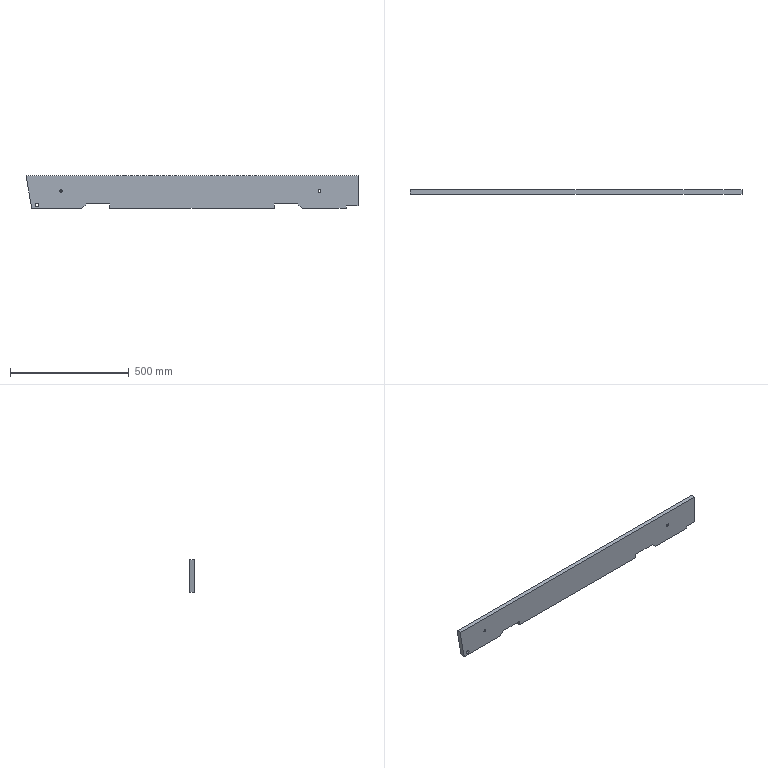Part | STEP file | Frame_right | 1 solid | 19 faces | box 1400 x 18 x 137 mm | volume 3336381 mm3 | plane 16 | cylinder 3 | commonest cylinder face diameters 11 x2 15 x1
STEP:
#1=CARTESIAN_POINT('',(0.,0.,0.));
#2=DIRECTION('',(0.,0.,1.));
#3=DIRECTION('',(1.,0.,0.));
#4=AXIS2_PLACEMENT_3D('',#1,#2,#3);
#5=CARTESIAN_POINT('',(-675.843,0.,-68.5));
#6=VERTEX_POINT('',#5);
#7=CARTESIAN_POINT('',(-464.5,0.,-68.5));
#8=VERTEX_POINT('',#7);
#9=CARTESIAN_POINT('',(-700.,0.,-68.5));
#10=DIRECTION('',(1.,0.,0.));
#11=VECTOR('',#10,1.);
#12=LINE('',#9,#11);
#13=CARTESIAN_POINT('',(-700.,0.,-68.5));
#14=DIRECTION('',(0.,0.,1.));
#15=DIRECTION('',(1.,0.,0.));
#16=AXIS2_PLACEMENT_3D('',#13,#14,#15);
#17=PLANE('',#16);
#18=CARTESIAN_POINT('',(0.,0.));
#19=DIRECTION('',(1.,0.));
#20=VECTOR('',#19,1.);
#21=LINE('',#18,#20);
#22=(GEOMETRIC_REPRESENTATION_CONTEXT(2)PARAMETRIC_REPRESENTATION_CONTEXT()REPRESENTATION_CONTEXT('',''));
#23=DEFINITIONAL_REPRESENTATION('',(#21),#22);
#24=PCURVE('',#17,#23);
#25=CARTESIAN_POINT('',(0.,0.,0.));
#26=DIRECTION('',(0.,1.,0.));
#27=DIRECTION('',(0.,0.,1.));
#28=AXIS2_PLACEMENT_3D('',#25,#26,#27);
#29=PLANE('',#28);
#30=CARTESIAN_POINT('',(-68.5,-700.));
#31=DIRECTION('',(0.,1.));
#32=VECTOR('',#31,1.);
#33=LINE('',#30,#32);
#34=(GEOMETRIC_REPRESENTATION_CONTEXT(2)PARAMETRIC_REPRESENTATION_CONTEXT()REPRESENTATION_CONTEXT('',''));
#35=DEFINITIONAL_REPRESENTATION('',(#33),#34);
#36=PCURVE('',#29,#35);
#37=SURFACE_CURVE('',#12,(#24,#36),.PCURVE_S1.);
#38=EDGE_CURVE('',#6,#8,#37,.T.);
#39=ORIENTED_EDGE('',*,*,#38,.F.);
#40=CARTESIAN_POINT('',(-675.843,-18.,-68.5));
#41=VERTEX_POINT('',#40);
#42=CARTESIAN_POINT('',(-675.843,0.,-68.5));
#43=DIRECTION('',(0.,-1.,0.));
#44=VECTOR('',#43,1.);
#45=LINE('',#42,#44);
#46=CARTESIAN_POINT('',(24.157,0.));
#47=DIRECTION('',(0.,-1.));
#48=VECTOR('',#47,1.);
#49=LINE('',#46,#48);
#50=(GEOMETRIC_REPRESENTATION_CONTEXT(2)PARAMETRIC_REPRESENTATION_CONTEXT()REPRESENTATION_CONTEXT('',''));
#51=DEFINITIONAL_REPRESENTATION('',(#49),#50);
#52=PCURVE('',#17,#51);
#53=CARTESIAN_POINT('',(-700.,0.,68.5));
#54=DIRECTION('',(0.9848,0.,0.1736));
#55=DIRECTION('',(0.1736,0.,-0.9848));
#56=AXIS2_PLACEMENT_3D('',#53,#54,#55);
#57=PLANE('',#56);
#58=CARTESIAN_POINT('',(139.113,0.));
#59=DIRECTION('',(0.,-1.));
#60=VECTOR('',#59,1.);
#61=LINE('',#58,#60);
#62=(GEOMETRIC_REPRESENTATION_CONTEXT(2)PARAMETRIC_REPRESENTATION_CONTEXT()REPRESENTATION_CONTEXT('',''));
#63=DEFINITIONAL_REPRESENTATION('',(#61),#62);
#64=PCURVE('',#57,#63);
#65=SURFACE_CURVE('',#45,(#52,#64),.PCURVE_S1.);
#66=EDGE_CURVE('',#6,#41,#65,.T.);
#67=ORIENTED_EDGE('',*,*,#66,.T.);
#68=CARTESIAN_POINT('',(-464.5,-18.,-68.5));
#69=VERTEX_POINT('',#68);
#70=CARTESIAN_POINT('',(-700.,-18.,-68.5));
#71=DIRECTION('',(1.,0.,0.));
#72=VECTOR('',#71,1.);
#73=LINE('',#70,#72);
#74=CARTESIAN_POINT('',(0.,-18.));
#75=DIRECTION('',(1.,0.));
#76=VECTOR('',#75,1.);
#77=LINE('',#74,#76);
#78=(GEOMETRIC_REPRESENTATION_CONTEXT(2)PARAMETRIC_REPRESENTATION_CONTEXT()REPRESENTATION_CONTEXT('',''));
#79=DEFINITIONAL_REPRESENTATION('',(#77),#78);
#80=PCURVE('',#17,#79);
#81=CARTESIAN_POINT('',(0.,-18.,0.));
#82=DIRECTION('',(0.,1.,0.));
#83=DIRECTION('',(0.,0.,1.));
#84=AXIS2_PLACEMENT_3D('',#81,#82,#83);
#85=PLANE('',#84);
#86=CARTESIAN_POINT('',(-68.5,-700.));
#87=DIRECTION('',(0.,1.));
#88=VECTOR('',#87,1.);
#89=LINE('',#86,#88);
#90=(GEOMETRIC_REPRESENTATION_CONTEXT(2)PARAMETRIC_REPRESENTATION_CONTEXT()REPRESENTATION_CONTEXT('',''));
#91=DEFINITIONAL_REPRESENTATION('',(#89),#90);
#92=PCURVE('',#85,#91);
#93=SURFACE_CURVE('',#73,(#80,#92),.PCURVE_S1.);
#94=EDGE_CURVE('',#41,#69,#93,.T.);
#95=ORIENTED_EDGE('',*,*,#94,.T.);
#96=CARTESIAN_POINT('',(-464.5,-18.,-68.5));
#97=DIRECTION('',(0.,1.,0.));
#98=VECTOR('',#97,1.);
#99=LINE('',#96,#98);
#100=CARTESIAN_POINT('',(235.5,-18.));
#101=DIRECTION('',(0.,1.));
#102=VECTOR('',#101,1.);
#103=LINE('',#100,#102);
#104=(GEOMETRIC_REPRESENTATION_CONTEXT(2)PARAMETRIC_REPRESENTATION_CONTEXT()REPRESENTATION_CONTEXT('',''));
#105=DEFINITIONAL_REPRESENTATION('',(#103),#104);
#106=PCURVE('',#17,#105);
#107=CARTESIAN_POINT('',(-446.5,-18.,-50.5));
#108=DIRECTION('',(-0.7071,0.,0.7071));
#109=DIRECTION('',(-0.7071,0.,-0.7071));
#110=AXIS2_PLACEMENT_3D('',#107,#108,#109);
#111=PLANE('',#110);
#112=CARTESIAN_POINT('',(25.456,0.));
#113=DIRECTION('',(0.,-1.));
#114=VECTOR('',#113,1.);
#115=LINE('',#112,#114);
#116=(GEOMETRIC_REPRESENTATION_CONTEXT(2)PARAMETRIC_REPRESENTATION_CONTEXT()REPRESENTATION_CONTEXT('',''));
#117=DEFINITIONAL_REPRESENTATION('',(#115),#116);
#118=PCURVE('',#111,#117);
#119=SURFACE_CURVE('',#99,(#106,#118),.PCURVE_S1.);
#120=EDGE_CURVE('',#69,#8,#119,.T.);
#121=ORIENTED_EDGE('',*,*,#120,.T.);
#122=EDGE_LOOP('',(#39,#67,#95,#121));
#123=FACE_BOUND('',#122,.F.);
#124=ADVANCED_FACE('',(#123),#17,.F.);
#125=ORIENTED_EDGE('',*,*,#38,.F.);
#126=CARTESIAN_POINT('',(-700.,0.,68.5));
#127=VERTEX_POINT('',#126);
#128=CARTESIAN_POINT('',(-683.589,0.,-24.571));
#129=DIRECTION('',(0.1736,0.,-0.9848));
#130=VECTOR('',#129,1.);
#131=LINE('',#128,#130);
#132=CARTESIAN_POINT('',(-24.571,-683.589));
#133=DIRECTION('',(-0.9848,0.1736));
#134=VECTOR('',#133,1.);
#135=LINE('',#132,#134);
#136=(GEOMETRIC_REPRESENTATION_CONTEXT(2)PARAMETRIC_REPRESENTATION_CONTEXT()REPRESENTATION_CONTEXT('',''));
#137=DEFINITIONAL_REPRESENTATION('',(#135),#136);
#138=PCURVE('',#29,#137);
#139=CARTESIAN_POINT('',(94.507,0.));
#140=DIRECTION('',(1.,0.));
#141=VECTOR('',#140,1.);
#142=LINE('',#139,#141);
#143=(GEOMETRIC_REPRESENTATION_CONTEXT(2)PARAMETRIC_REPRESENTATION_CONTEXT()REPRESENTATION_CONTEXT('',''));
#144=DEFINITIONAL_REPRESENTATION('',(#142),#143);
#145=PCURVE('',#57,#144);
#146=SURFACE_CURVE('',#131,(#138,#145),.PCURVE_S1.);
#147=EDGE_CURVE('',#127,#6,#146,.T.);
#148=ORIENTED_EDGE('',*,*,#147,.F.);
#149=CARTESIAN_POINT('',(700.,0.,68.5));
#150=VERTEX_POINT('',#149);
#151=CARTESIAN_POINT('',(700.,0.,68.5));
#152=DIRECTION('',(-1.,0.,0.));
#153=VECTOR('',#152,1.);
#154=LINE('',#151,#153);
#155=CARTESIAN_POINT('',(68.5,700.));
#156=DIRECTION('',(0.,-1.));
#157=VECTOR('',#156,1.);
#158=LINE('',#155,#157);
#159=(GEOMETRIC_REPRESENTATION_CONTEXT(2)PARAMETRIC_REPRESENTATION_CONTEXT()REPRESENTATION_CONTEXT('',''));
#160=DEFINITIONAL_REPRESENTATION('',(#158),#159);
#161=PCURVE('',#29,#160);
#162=CARTESIAN_POINT('',(700.,0.,68.5));
#163=DIRECTION('',(0.,0.,-1.));
#164=DIRECTION('',(-1.,0.,0.));
#165=AXIS2_PLACEMENT_3D('',#162,#163,#164);
#166=PLANE('',#165);
#167=CARTESIAN_POINT('',(0.,0.));
#168=DIRECTION('',(1.,0.));
#169=VECTOR('',#168,1.);
#170=LINE('',#167,#169);
#171=(GEOMETRIC_REPRESENTATION_CONTEXT(2)PARAMETRIC_REPRESENTATION_CONTEXT()REPRESENTATION_CONTEXT('',''));
#172=DEFINITIONAL_REPRESENTATION('',(#170),#171);
#173=PCURVE('',#166,#172);
#174=SURFACE_CURVE('',#154,(#161,#173),.PCURVE_S1.);
#175=EDGE_CURVE('',#150,#127,#174,.T.);
#176=ORIENTED_EDGE('',*,*,#175,.F.);
#177=CARTESIAN_POINT('',(700.,0.,-58.5));
#178=VERTEX_POINT('',#177);
#179=CARTESIAN_POINT('',(700.,0.,-68.5));
#180=DIRECTION('',(0.,0.,1.));
#181=VECTOR('',#180,1.);
#182=LINE('',#179,#181);
#183=CARTESIAN_POINT('',(-68.5,700.));
#184=DIRECTION('',(1.,0.));
#185=VECTOR('',#184,1.);
#186=LINE('',#183,#185);
#187=(GEOMETRIC_REPRESENTATION_CONTEXT(2)PARAMETRIC_REPRESENTATION_CONTEXT()REPRESENTATION_CONTEXT('',''));
#188=DEFINITIONAL_REPRESENTATION('',(#186),#187);
#189=PCURVE('',#29,#188);
#190=CARTESIAN_POINT('',(700.,0.,-68.5));
#191=DIRECTION('',(-1.,0.,0.));
#192=DIRECTION('',(0.,0.,1.));
#193=AXIS2_PLACEMENT_3D('',#190,#191,#192);
#194=PLANE('',#193);
#195=CARTESIAN_POINT('',(0.,0.));
#196=DIRECTION('',(1.,0.));
#197=VECTOR('',#196,1.);
#198=LINE('',#195,#197);
#199=(GEOMETRIC_REPRESENTATION_CONTEXT(2)PARAMETRIC_REPRESENTATION_CONTEXT()REPRESENTATION_CONTEXT('',''));
#200=DEFINITIONAL_REPRESENTATION('',(#198),#199);
#201=PCURVE('',#194,#200);
#202=SURFACE_CURVE('',#182,(#189,#201),.PCURVE_S1.);
#203=EDGE_CURVE('',#178,#150,#202,.T.);
#204=ORIENTED_EDGE('',*,*,#203,.F.);
#205=CARTESIAN_POINT('',(650.,0.,-58.5));
#206=VERTEX_POINT('',#205);
#207=CARTESIAN_POINT('',(350.,0.,-58.5));
#208=DIRECTION('',(1.,0.,0.));
#209=VECTOR('',#208,1.);
#210=LINE('',#207,#209);
#211=CARTESIAN_POINT('',(-58.5,350.));
#212=DIRECTION('',(0.,1.));
#213=VECTOR('',#212,1.);
#214=LINE('',#211,#213);
#215=(GEOMETRIC_REPRESENTATION_CONTEXT(2)PARAMETRIC_REPRESENTATION_CONTEXT()REPRESENTATION_CONTEXT('',''));
#216=DEFINITIONAL_REPRESENTATION('',(#214),#215);
#217=PCURVE('',#29,#216);
#218=CARTESIAN_POINT('',(700.,-18.,-58.5));
#219=DIRECTION('',(0.,0.,1.));
#220=DIRECTION('',(-1.,0.,0.));
#221=AXIS2_PLACEMENT_3D('',#218,#219,#220);
#222=PLANE('',#221);
#223=CARTESIAN_POINT('',(350.,-18.));
#224=DIRECTION('',(-1.,0.));
#225=VECTOR('',#224,1.);
#226=LINE('',#223,#225);
#227=(GEOMETRIC_REPRESENTATION_CONTEXT(2)PARAMETRIC_REPRESENTATION_CONTEXT()REPRESENTATION_CONTEXT('',''));
#228=DEFINITIONAL_REPRESENTATION('',(#226),#227);
#229=PCURVE('',#222,#228);
#230=SURFACE_CURVE('',#210,(#217,#229),.PCURVE_S1.);
#231=EDGE_CURVE('',#206,#178,#230,.T.);
#232=ORIENTED_EDGE('',*,*,#231,.F.);
#233=CARTESIAN_POINT('',(650.,0.,-68.5));
#234=VERTEX_POINT('',#233);
#235=CARTESIAN_POINT('',(650.,0.,-29.25));
#236=DIRECTION('',(0.,0.,1.));
#237=VECTOR('',#236,1.);
#238=LINE('',#235,#237);
#239=CARTESIAN_POINT('',(-29.25,650.));
#240=DIRECTION('',(1.,0.));
#241=VECTOR('',#240,1.);
#242=LINE('',#239,#241);
#243=(GEOMETRIC_REPRESENTATION_CONTEXT(2)PARAMETRIC_REPRESENTATION_CONTEXT()REPRESENTATION_CONTEXT('',''));
#244=DEFINITIONAL_REPRESENTATION('',(#242),#243);
#245=PCURVE('',#29,#244);
#246=CARTESIAN_POINT('',(650.,-18.,-58.5));
#247=DIRECTION('',(-1.,0.,0.));
#248=DIRECTION('',(0.,0.,-1.));
#249=AXIS2_PLACEMENT_3D('',#246,#247,#248);
#250=PLANE('',#249);
#251=CARTESIAN_POINT('',(-29.25,-18.));
#252=DIRECTION('',(-1.,0.));
#253=VECTOR('',#252,1.);
#254=LINE('',#251,#253);
#255=(GEOMETRIC_REPRESENTATION_CONTEXT(2)PARAMETRIC_REPRESENTATION_CONTEXT()REPRESENTATION_CONTEXT('',''));
#256=DEFINITIONAL_REPRESENTATION('',(#254),#255);
#257=PCURVE('',#250,#256);
#258=SURFACE_CURVE('',#238,(#245,#257),.PCURVE_S1.);
#259=EDGE_CURVE('',#234,#206,#258,.T.);
#260=ORIENTED_EDGE('',*,*,#259,.F.);
#261=CARTESIAN_POINT('',(464.5,0.,-68.5));
#262=VERTEX_POINT('',#261);
#263=CARTESIAN_POINT('',(-700.,0.,-68.5));
#264=DIRECTION('',(1.,0.,0.));
#265=VECTOR('',#264,1.);
#266=LINE('',#263,#265);
#267=CARTESIAN_POINT('',(-68.5,-700.));
#268=DIRECTION('',(0.,1.));
#269=VECTOR('',#268,1.);
#270=LINE('',#267,#269);
#271=(GEOMETRIC_REPRESENTATION_CONTEXT(2)PARAMETRIC_REPRESENTATION_CONTEXT()REPRESENTATION_CONTEXT('',''));
#272=DEFINITIONAL_REPRESENTATION('',(#270),#271);
#273=PCURVE('',#29,#272);
#274=CARTESIAN_POINT('',(-700.,0.,-68.5));
#275=DIRECTION('',(0.,0.,1.));
#276=DIRECTION('',(1.,0.,0.));
#277=AXIS2_PLACEMENT_3D('',#274,#275,#276);
#278=PLANE('',#277);
#279=CARTESIAN_POINT('',(0.,0.));
#280=DIRECTION('',(1.,0.));
#281=VECTOR('',#280,1.);
#282=LINE('',#279,#281);
#283=(GEOMETRIC_REPRESENTATION_CONTEXT(2)PARAMETRIC_REPRESENTATION_CONTEXT()REPRESENTATION_CONTEXT('',''));
#284=DEFINITIONAL_REPRESENTATION('',(#282),#283);
#285=PCURVE('',#278,#284);
#286=SURFACE_CURVE('',#266,(#273,#285),.PCURVE_S1.);
#287=EDGE_CURVE('',#262,#234,#286,.T.);
#288=ORIENTED_EDGE('',*,*,#287,.F.);
#289=CARTESIAN_POINT('',(446.5,0.,-50.5));
#290=VERTEX_POINT('',#289);
#291=CARTESIAN_POINT('',(322.25,0.,73.75));
#292=DIRECTION('',(-0.7071,0.,0.7071));
#293=VECTOR('',#292,1.);
#294=LINE('',#291,#293);
#295=CARTESIAN_POINT('',(73.75,322.25));
#296=DIRECTION('',(0.7071,-0.7071));
#297=VECTOR('',#296,1.);
#298=LINE('',#295,#297);
#299=(GEOMETRIC_REPRESENTATION_CONTEXT(2)PARAMETRIC_REPRESENTATION_CONTEXT()REPRESENTATION_CONTEXT('',''));
#300=DEFINITIONAL_REPRESENTATION('',(#298),#299);
#301=PCURVE('',#29,#300);
#302=CARTESIAN_POINT('',(446.5,-18.,-50.5));
#303=DIRECTION('',(-0.7071,0.,-0.7071));
#304=DIRECTION('',(0.7071,0.,-0.7071));
#305=AXIS2_PLACEMENT_3D('',#302,#303,#304);
#306=PLANE('',#305);
#307=CARTESIAN_POINT('',(-175.716,-18.));
#308=DIRECTION('',(-1.,0.));
#309=VECTOR('',#308,1.);
#310=LINE('',#307,#309);
#311=(GEOMETRIC_REPRESENTATION_CONTEXT(2)PARAMETRIC_REPRESENTATION_CONTEXT()REPRESENTATION_CONTEXT('',''));
#312=DEFINITIONAL_REPRESENTATION('',(#310),#311);
#313=PCURVE('',#306,#312);
#314=SURFACE_CURVE('',#294,(#301,#313),.PCURVE_S1.);
#315=EDGE_CURVE('',#262,#290,#314,.T.);
#316=ORIENTED_EDGE('',*,*,#315,.T.);
#317=CARTESIAN_POINT('',(346.5,0.,-50.5));
#318=VERTEX_POINT('',#317);
#319=CARTESIAN_POINT('',(173.25,0.,-50.5));
#320=DIRECTION('',(-1.,0.,0.));
#321=VECTOR('',#320,1.);
#322=LINE('',#319,#321);
#323=CARTESIAN_POINT('',(-50.5,173.25));
#324=DIRECTION('',(0.,-1.));
#325=VECTOR('',#324,1.);
#326=LINE('',#323,#325);
#327=(GEOMETRIC_REPRESENTATION_CONTEXT(2)PARAMETRIC_REPRESENTATION_CONTEXT()REPRESENTATION_CONTEXT('',''));
#328=DEFINITIONAL_REPRESENTATION('',(#326),#327);
#329=PCURVE('',#29,#328);
#330=CARTESIAN_POINT('',(346.5,-18.,-50.5));
#331=DIRECTION('',(0.,0.,-1.));
#332=DIRECTION('',(1.,0.,0.));
#333=AXIS2_PLACEMENT_3D('',#330,#331,#332);
#334=PLANE('',#333);
#335=CARTESIAN_POINT('',(-173.25,-18.));
#336=DIRECTION('',(-1.,0.));
#337=VECTOR('',#336,1.);
#338=LINE('',#335,#337);
#339=(GEOMETRIC_REPRESENTATION_CONTEXT(2)PARAMETRIC_REPRESENTATION_CONTEXT()REPRESENTATION_CONTEXT('',''));
#340=DEFINITIONAL_REPRESENTATION('',(#338),#339);
#341=PCURVE('',#334,#340);
#342=SURFACE_CURVE('',#322,(#329,#341),.PCURVE_S1.);
#343=EDGE_CURVE('',#290,#318,#342,.T.);
#344=ORIENTED_EDGE('',*,*,#343,.T.);
#345=CARTESIAN_POINT('',(346.5,0.,-68.5));
#346=VERTEX_POINT('',#345);
#347=CARTESIAN_POINT('',(346.5,0.,-34.25));
#348=DIRECTION('',(0.,0.,-1.));
#349=VECTOR('',#348,1.);
#350=LINE('',#347,#349);
#351=CARTESIAN_POINT('',(-34.25,346.5));
#352=DIRECTION('',(-1.,0.));
#353=VECTOR('',#352,1.);
#354=LINE('',#351,#353);
#355=(GEOMETRIC_REPRESENTATION_CONTEXT(2)PARAMETRIC_REPRESENTATION_CONTEXT()REPRESENTATION_CONTEXT('',''));
#356=DEFINITIONAL_REPRESENTATION('',(#354),#355);
#357=PCURVE('',#29,#356);
#358=CARTESIAN_POINT('',(346.5,-18.,-68.5));
#359=DIRECTION('',(1.,0.,0.));
#360=DIRECTION('',(0.,0.,1.));
#361=AXIS2_PLACEMENT_3D('',#358,#359,#360);
#362=PLANE('',#361);
#363=CARTESIAN_POINT('',(34.25,-18.));
#364=DIRECTION('',(-1.,0.));
#365=VECTOR('',#364,1.);
#366=LINE('',#363,#365);
#367=(GEOMETRIC_REPRESENTATION_CONTEXT(2)PARAMETRIC_REPRESENTATION_CONTEXT()REPRESENTATION_CONTEXT('',''));
#368=DEFINITIONAL_REPRESENTATION('',(#366),#367);
#369=PCURVE('',#362,#368);
#370=SURFACE_CURVE('',#350,(#357,#369),.PCURVE_S1.);
#371=EDGE_CURVE('',#318,#346,#370,.T.);
#372=ORIENTED_EDGE('',*,*,#371,.T.);
#373=CARTESIAN_POINT('',(-346.5,0.,-68.5));
#374=VERTEX_POINT('',#373);
#375=CARTESIAN_POINT('',(-700.,0.,-68.5));
#376=DIRECTION('',(1.,0.,0.));
#377=VECTOR('',#376,1.);
#378=LINE('',#375,#377);
#379=CARTESIAN_POINT('',(-68.5,-700.));
#380=DIRECTION('',(0.,1.));
#381=VECTOR('',#380,1.);
#382=LINE('',#379,#381);
#383=(GEOMETRIC_REPRESENTATION_CONTEXT(2)PARAMETRIC_REPRESENTATION_CONTEXT()REPRESENTATION_CONTEXT('',''));
#384=DEFINITIONAL_REPRESENTATION('',(#382),#383);
#385=PCURVE('',#29,#384);
#386=CARTESIAN_POINT('',(-700.,0.,-68.5));
#387=DIRECTION('',(0.,0.,1.));
#388=DIRECTION('',(1.,0.,0.));
#389=AXIS2_PLACEMENT_3D('',#386,#387,#388);
#390=PLANE('',#389);
#391=CARTESIAN_POINT('',(0.,0.));
#392=DIRECTION('',(1.,0.));
#393=VECTOR('',#392,1.);
#394=LINE('',#391,#393);
#395=(GEOMETRIC_REPRESENTATION_CONTEXT(2)PARAMETRIC_REPRESENTATION_CONTEXT()REPRESENTATION_CONTEXT('',''));
#396=DEFINITIONAL_REPRESENTATION('',(#394),#395);
#397=PCURVE('',#390,#396);
#398=SURFACE_CURVE('',#378,(#385,#397),.PCURVE_S1.);
#399=EDGE_CURVE('',#374,#346,#398,.T.);
#400=ORIENTED_EDGE('',*,*,#399,.F.);
#401=CARTESIAN_POINT('',(-346.5,0.,-50.5));
#402=VERTEX_POINT('',#401);
#403=CARTESIAN_POINT('',(-346.5,0.,-34.25));
#404=DIRECTION('',(0.,0.,-1.));
#405=VECTOR('',#404,1.);
#406=LINE('',#403,#405);
#407=CARTESIAN_POINT('',(-34.25,-346.5));
#408=DIRECTION('',(-1.,0.));
#409=VECTOR('',#408,1.);
#410=LINE('',#407,#409);
#411=(GEOMETRIC_REPRESENTATION_CONTEXT(2)PARAMETRIC_REPRESENTATION_CONTEXT()REPRESENTATION_CONTEXT('',''));
#412=DEFINITIONAL_REPRESENTATION('',(#410),#411);
#413=PCURVE('',#29,#412);
#414=CARTESIAN_POINT('',(-346.5,-18.,-68.5));
#415=DIRECTION('',(1.,0.,0.));
#416=DIRECTION('',(0.,0.,1.));
#417=AXIS2_PLACEMENT_3D('',#414,#415,#416);
#418=PLANE('',#417);
#419=CARTESIAN_POINT('',(34.25,-18.));
#420=DIRECTION('',(-1.,0.));
#421=VECTOR('',#420,1.);
#422=LINE('',#419,#421);
#423=(GEOMETRIC_REPRESENTATION_CONTEXT(2)PARAMETRIC_REPRESENTATION_CONTEXT()REPRESENTATION_CONTEXT('',''));
#424=DEFINITIONAL_REPRESENTATION('',(#422),#423);
#425=PCURVE('',#418,#424);
#426=SURFACE_CURVE('',#406,(#413,#425),.PCURVE_S1.);
#427=EDGE_CURVE('',#402,#374,#426,.T.);
#428=ORIENTED_EDGE('',*,*,#427,.F.);
#429=CARTESIAN_POINT('',(-446.5,0.,-50.5));
#430=VERTEX_POINT('',#429);
#431=CARTESIAN_POINT('',(-173.25,0.,-50.5));
#432=DIRECTION('',(1.,0.,0.));
#433=VECTOR('',#432,1.);
#434=LINE('',#431,#433);
#435=CARTESIAN_POINT('',(-50.5,-173.25));
#436=DIRECTION('',(0.,1.));
#437=VECTOR('',#436,1.);
#438=LINE('',#435,#437);
#439=(GEOMETRIC_REPRESENTATION_CONTEXT(2)PARAMETRIC_REPRESENTATION_CONTEXT()REPRESENTATION_CONTEXT('',''));
#440=DEFINITIONAL_REPRESENTATION('',(#438),#439);
#441=PCURVE('',#29,#440);
#442=CARTESIAN_POINT('',(-346.5,-18.,-50.5));
#443=DIRECTION('',(0.,0.,1.));
#444=DIRECTION('',(-1.,0.,0.));
#445=AXIS2_PLACEMENT_3D('',#442,#443,#444);
#446=PLANE('',#445);
#447=CARTESIAN_POINT('',(-173.25,-18.));
#448=DIRECTION('',(-1.,0.));
#449=VECTOR('',#448,1.);
#450=LINE('',#447,#449);
#451=(GEOMETRIC_REPRESENTATION_CONTEXT(2)PARAMETRIC_REPRESENTATION_CONTEXT()REPRESENTATION_CONTEXT('',''));
#452=DEFINITIONAL_REPRESENTATION('',(#450),#451);
#453=PCURVE('',#446,#452);
#454=SURFACE_CURVE('',#434,(#441,#453),.PCURVE_S1.);
#455=EDGE_CURVE('',#430,#402,#454,.T.);
#456=ORIENTED_EDGE('',*,*,#455,.F.);
#457=CARTESIAN_POINT('',(-322.25,0.,73.75));
#458=DIRECTION('',(0.7071,0.,0.7071));
#459=VECTOR('',#458,1.);
#460=LINE('',#457,#459);
#461=CARTESIAN_POINT('',(73.75,-322.25));
#462=DIRECTION('',(0.7071,0.7071));
#463=VECTOR('',#462,1.);
#464=LINE('',#461,#463);
#465=(GEOMETRIC_REPRESENTATION_CONTEXT(2)PARAMETRIC_REPRESENTATION_CONTEXT()REPRESENTATION_CONTEXT('',''));
#466=DEFINITIONAL_REPRESENTATION('',(#464),#465);
#467=PCURVE('',#29,#466);
#468=CARTESIAN_POINT('',(-175.716,-18.));
#469=DIRECTION('',(-1.,0.));
#470=VECTOR('',#469,1.);
#471=LINE('',#468,#470);
#472=(GEOMETRIC_REPRESENTATION_CONTEXT(2)PARAMETRIC_REPRESENTATION_CONTEXT()REPRESENTATION_CONTEXT('',''));
#473=DEFINITIONAL_REPRESENTATION('',(#471),#472);
#474=PCURVE('',#111,#473);
#475=SURFACE_CURVE('',#460,(#467,#474),.PCURVE_S1.);
#476=EDGE_CURVE('',#8,#430,#475,.T.);
#477=ORIENTED_EDGE('',*,*,#476,.F.);
#478=EDGE_LOOP('',(#125,#148,#176,#204,#232,#260,#288,#316,#344,#372,#400,#428,#456,#477));
#479=FACE_BOUND('',#478,.T.);
#480=CARTESIAN_POINT('',(-661.343,0.,-55.5));
#481=VERTEX_POINT('',#480);
#482=CARTESIAN_POINT('',(-653.843,0.,-55.5));
#483=DIRECTION('',(0.,1.,0.));
#484=DIRECTION('',(-1.,0.,0.));
#485=AXIS2_PLACEMENT_3D('',#482,#483,#484);
#486=CIRCLE('',#485,7.5);
#487=CARTESIAN_POINT('',(-55.5,-653.843));
#488=DIRECTION('',(0.,-1.));
#489=AXIS2_PLACEMENT_2D('',#487,#488);
#490=CIRCLE('',#489,7.5);
#491=(GEOMETRIC_REPRESENTATION_CONTEXT(2)PARAMETRIC_REPRESENTATION_CONTEXT()REPRESENTATION_CONTEXT('',''));
#492=DEFINITIONAL_REPRESENTATION('',(#490),#491);
#493=PCURVE('',#29,#492);
#494=CARTESIAN_POINT('',(-653.843,-18.,-55.5));
#495=DIRECTION('',(0.,1.,0.));
#496=DIRECTION('',(-1.,0.,0.));
#497=AXIS2_PLACEMENT_3D('',#494,#495,#496);
#498=CYLINDRICAL_SURFACE('',#497,7.5);
#499=CARTESIAN_POINT('',(0.,18.));
#500=DIRECTION('',(1.,0.));
#501=VECTOR('',#500,1.);
#502=LINE('',#499,#501);
#503=(GEOMETRIC_REPRESENTATION_CONTEXT(2)PARAMETRIC_REPRESENTATION_CONTEXT()REPRESENTATION_CONTEXT('',''));
#504=DEFINITIONAL_REPRESENTATION('',(#502),#503);
#505=PCURVE('',#498,#504);
#506=SURFACE_CURVE('',#486,(#493,#505),.PCURVE_S1.);
#507=EDGE_CURVE('',#481,#481,#506,.T.);
#508=ORIENTED_EDGE('',*,*,#507,.F.);
#509=EDGE_LOOP('',(#508));
#510=FACE_BOUND('',#509,.T.);
#511=CARTESIAN_POINT('',(-557.9,0.,4.5));
#512=VERTEX_POINT('',#511);
#513=CARTESIAN_POINT('',(-552.4,0.,4.5));
#514=DIRECTION('',(0.,1.,0.));
#515=DIRECTION('',(-1.,0.,0.));
#516=AXIS2_PLACEMENT_3D('',#513,#514,#515);
#517=CIRCLE('',#516,5.5);
#518=CARTESIAN_POINT('',(4.5,-552.4));
#519=DIRECTION('',(0.,-1.));
#520=AXIS2_PLACEMENT_2D('',#518,#519);
#521=CIRCLE('',#520,5.5);
#522=(GEOMETRIC_REPRESENTATION_CONTEXT(2)PARAMETRIC_REPRESENTATION_CONTEXT()REPRESENTATION_CONTEXT('',''));
#523=DEFINITIONAL_REPRESENTATION('',(#521),#522);
#524=PCURVE('',#29,#523);
#525=CARTESIAN_POINT('',(-552.4,-18.,4.5));
#526=DIRECTION('',(0.,1.,0.));
#527=DIRECTION('',(-1.,0.,0.));
#528=AXIS2_PLACEMENT_3D('',#525,#526,#527);
#529=CYLINDRICAL_SURFACE('',#528,5.5);
#530=CARTESIAN_POINT('',(0.,18.));
#531=DIRECTION('',(1.,0.));
#532=VECTOR('',#531,1.);
#533=LINE('',#530,#532);
#534=(GEOMETRIC_REPRESENTATION_CONTEXT(2)PARAMETRIC_REPRESENTATION_CONTEXT()REPRESENTATION_CONTEXT('',''));
#535=DEFINITIONAL_REPRESENTATION('',(#533),#534);
#536=PCURVE('',#529,#535);
#537=SURFACE_CURVE('',#517,(#524,#536),.PCURVE_S1.);
#538=EDGE_CURVE('',#512,#512,#537,.T.);
#539=ORIENTED_EDGE('',*,*,#538,.F.);
#540=EDGE_LOOP('',(#539));
#541=FACE_BOUND('',#540,.T.);
#542=CARTESIAN_POINT('',(531.7,0.,4.5));
#543=VERTEX_POINT('',#542);
#544=CARTESIAN_POINT('',(537.2,0.,4.5));
#545=DIRECTION('',(0.,1.,0.));
#546=DIRECTION('',(-1.,0.,0.));
#547=AXIS2_PLACEMENT_3D('',#544,#545,#546);
#548=CIRCLE('',#547,5.5);
#549=CARTESIAN_POINT('',(4.5,537.2));
#550=DIRECTION('',(0.,-1.));
#551=AXIS2_PLACEMENT_2D('',#549,#550);
#552=CIRCLE('',#551,5.5);
#553=(GEOMETRIC_REPRESENTATION_CONTEXT(2)PARAMETRIC_REPRESENTATION_CONTEXT()REPRESENTATION_CONTEXT('',''));
#554=DEFINITIONAL_REPRESENTATION('',(#552),#553);
#555=PCURVE('',#29,#554);
#556=CARTESIAN_POINT('',(537.2,-18.,4.5));
#557=DIRECTION('',(0.,1.,0.));
#558=DIRECTION('',(-1.,0.,0.));
#559=AXIS2_PLACEMENT_3D('',#556,#557,#558);
#560=CYLINDRICAL_SURFACE('',#559,5.5);
#561=CARTESIAN_POINT('',(0.,18.));
#562=DIRECTION('',(1.,0.));
#563=VECTOR('',#562,1.);
#564=LINE('',#561,#563);
#565=(GEOMETRIC_REPRESENTATION_CONTEXT(2)PARAMETRIC_REPRESENTATION_CONTEXT()REPRESENTATION_CONTEXT('',''));
#566=DEFINITIONAL_REPRESENTATION('',(#564),#565);
#567=PCURVE('',#560,#566);
#568=SURFACE_CURVE('',#548,(#555,#567),.PCURVE_S1.);
#569=EDGE_CURVE('',#543,#543,#568,.T.);
#570=ORIENTED_EDGE('',*,*,#569,.F.);
#571=EDGE_LOOP('',(#570));
#572=FACE_BOUND('',#571,.T.);
#573=ADVANCED_FACE('',(#479,#510,#541,#572),#29,.T.);
#574=CARTESIAN_POINT('',(-446.5,-18.,-50.5));
#575=VERTEX_POINT('',#574);
#576=CARTESIAN_POINT('',(-446.5,-18.,-50.5));
#577=DIRECTION('',(-0.7071,0.,-0.7071));
#578=VECTOR('',#577,1.);
#579=LINE('',#576,#578);
#580=CARTESIAN_POINT('',(0.,0.));
#581=DIRECTION('',(1.,0.));
#582=VECTOR('',#581,1.);
#583=LINE('',#580,#582);
#584=(GEOMETRIC_REPRESENTATION_CONTEXT(2)PARAMETRIC_REPRESENTATION_CONTEXT()REPRESENTATION_CONTEXT('',''));
#585=DEFINITIONAL_REPRESENTATION('',(#583),#584);
#586=PCURVE('',#111,#585);
#587=CARTESIAN_POINT('',(-50.5,-446.5));
#588=DIRECTION('',(-0.7071,-0.7071));
#589=VECTOR('',#588,1.);
#590=LINE('',#587,#589);
#591=(GEOMETRIC_REPRESENTATION_CONTEXT(2)PARAMETRIC_REPRESENTATION_CONTEXT()REPRESENTATION_CONTEXT('',''));
#592=DEFINITIONAL_REPRESENTATION('',(#590),#591);
#593=PCURVE('',#85,#592);
#594=SURFACE_CURVE('',#579,(#586,#593),.PCURVE_S1.);
#595=EDGE_CURVE('',#575,#69,#594,.T.);
#596=ORIENTED_EDGE('',*,*,#595,.F.);
#597=CARTESIAN_POINT('',(-446.5,-18.,-50.5));
#598=DIRECTION('',(0.,1.,0.));
#599=VECTOR('',#598,1.);
#600=LINE('',#597,#599);
#601=CARTESIAN_POINT('',(0.,0.));
#602=DIRECTION('',(0.,-1.));
#603=VECTOR('',#602,1.);
#604=LINE('',#601,#603);
#605=(GEOMETRIC_REPRESENTATION_CONTEXT(2)PARAMETRIC_REPRESENTATION_CONTEXT()REPRESENTATION_CONTEXT('',''));
#606=DEFINITIONAL_REPRESENTATION('',(#604),#605);
#607=PCURVE('',#111,#606);
#608=CARTESIAN_POINT('',(100.,0.));
#609=DIRECTION('',(0.,-1.));
#610=VECTOR('',#609,1.);
#611=LINE('',#608,#610);
#612=(GEOMETRIC_REPRESENTATION_CONTEXT(2)PARAMETRIC_REPRESENTATION_CONTEXT()REPRESENTATION_CONTEXT('',''));
#613=DEFINITIONAL_REPRESENTATION('',(#611),#612);
#614=PCURVE('',#446,#613);
#615=SURFACE_CURVE('',#600,(#607,#614),.PCURVE_S1.);
#616=EDGE_CURVE('',#575,#430,#615,.T.);
#617=ORIENTED_EDGE('',*,*,#616,.T.);
#618=ORIENTED_EDGE('',*,*,#476,.F.);
#619=ORIENTED_EDGE('',*,*,#120,.F.);
#620=EDGE_LOOP('',(#596,#617,#618,#619));
#621=FACE_BOUND('',#620,.F.);
#622=ADVANCED_FACE('',(#621),#111,.F.);
#623=ORIENTED_EDGE('',*,*,#94,.F.);
#624=CARTESIAN_POINT('',(-700.,-18.,68.5));
#625=VERTEX_POINT('',#624);
#626=CARTESIAN_POINT('',(-683.589,-18.,-24.571));
#627=DIRECTION('',(0.1736,0.,-0.9848));
#628=VECTOR('',#627,1.);
#629=LINE('',#626,#628);
#630=CARTESIAN_POINT('',(-24.571,-683.589));
#631=DIRECTION('',(-0.9848,0.1736));
#632=VECTOR('',#631,1.);
#633=LINE('',#630,#632);
#634=(GEOMETRIC_REPRESENTATION_CONTEXT(2)PARAMETRIC_REPRESENTATION_CONTEXT()REPRESENTATION_CONTEXT('',''));
#635=DEFINITIONAL_REPRESENTATION('',(#633),#634);
#636=PCURVE('',#85,#635);
#637=CARTESIAN_POINT('',(94.507,-18.));
#638=DIRECTION('',(1.,0.));
#639=VECTOR('',#638,1.);
#640=LINE('',#637,#639);
#641=(GEOMETRIC_REPRESENTATION_CONTEXT(2)PARAMETRIC_REPRESENTATION_CONTEXT()REPRESENTATION_CONTEXT('',''));
#642=DEFINITIONAL_REPRESENTATION('',(#640),#641);
#643=PCURVE('',#57,#642);
#644=SURFACE_CURVE('',#629,(#636,#643),.PCURVE_S1.);
#645=EDGE_CURVE('',#625,#41,#644,.T.);
#646=ORIENTED_EDGE('',*,*,#645,.F.);
#647=CARTESIAN_POINT('',(700.,-18.,68.5));
#648=VERTEX_POINT('',#647);
#649=CARTESIAN_POINT('',(700.,-18.,68.5));
#650=DIRECTION('',(-1.,0.,0.));
#651=VECTOR('',#650,1.);
#652=LINE('',#649,#651);
#653=CARTESIAN_POINT('',(68.5,700.));
#654=DIRECTION('',(0.,-1.));
#655=VECTOR('',#654,1.);
#656=LINE('',#653,#655);
#657=(GEOMETRIC_REPRESENTATION_CONTEXT(2)PARAMETRIC_REPRESENTATION_CONTEXT()REPRESENTATION_CONTEXT('',''));
#658=DEFINITIONAL_REPRESENTATION('',(#656),#657);
#659=PCURVE('',#85,#658);
#660=CARTESIAN_POINT('',(0.,-18.));
#661=DIRECTION('',(1.,0.));
#662=VECTOR('',#661,1.);
#663=LINE('',#660,#662);
#664=(GEOMETRIC_REPRESENTATION_CONTEXT(2)PARAMETRIC_REPRESENTATION_CONTEXT()REPRESENTATION_CONTEXT('',''));
#665=DEFINITIONAL_REPRESENTATION('',(#663),#664);
#666=PCURVE('',#166,#665);
#667=SURFACE_CURVE('',#652,(#659,#666),.PCURVE_S1.);
#668=EDGE_CURVE('',#648,#625,#667,.T.);
#669=ORIENTED_EDGE('',*,*,#668,.F.);
#670=CARTESIAN_POINT('',(700.,-18.,-58.5));
#671=VERTEX_POINT('',#670);
#672=CARTESIAN_POINT('',(700.,-18.,-68.5));
#673=DIRECTION('',(0.,0.,1.));
#674=VECTOR('',#673,1.);
#675=LINE('',#672,#674);
#676=CARTESIAN_POINT('',(-68.5,700.));
#677=DIRECTION('',(1.,0.));
#678=VECTOR('',#677,1.);
#679=LINE('',#676,#678);
#680=(GEOMETRIC_REPRESENTATION_CONTEXT(2)PARAMETRIC_REPRESENTATION_CONTEXT()REPRESENTATION_CONTEXT('',''));
#681=DEFINITIONAL_REPRESENTATION('',(#679),#680);
#682=PCURVE('',#85,#681);
#683=CARTESIAN_POINT('',(0.,-18.));
#684=DIRECTION('',(1.,0.));
#685=VECTOR('',#684,1.);
#686=LINE('',#683,#685);
#687=(GEOMETRIC_REPRESENTATION_CONTEXT(2)PARAMETRIC_REPRESENTATION_CONTEXT()REPRESENTATION_CONTEXT('',''));
#688=DEFINITIONAL_REPRESENTATION('',(#686),#687);
#689=PCURVE('',#194,#688);
#690=SURFACE_CURVE('',#675,(#682,#689),.PCURVE_S1.);
#691=EDGE_CURVE('',#671,#648,#690,.T.);
#692=ORIENTED_EDGE('',*,*,#691,.F.);
#693=CARTESIAN_POINT('',(650.,-18.,-58.5));
#694=VERTEX_POINT('',#693);
#695=CARTESIAN_POINT('',(700.,-18.,-58.5));
#696=DIRECTION('',(-1.,0.,0.));
#697=VECTOR('',#696,1.);
#698=LINE('',#695,#697);
#699=CARTESIAN_POINT('',(-58.5,700.));
#700=DIRECTION('',(0.,-1.));
#701=VECTOR('',#700,1.);
#702=LINE('',#699,#701);
#703=(GEOMETRIC_REPRESENTATION_CONTEXT(2)PARAMETRIC_REPRESENTATION_CONTEXT()REPRESENTATION_CONTEXT('',''));
#704=DEFINITIONAL_REPRESENTATION('',(#702),#703);
#705=PCURVE('',#85,#704);
#706=CARTESIAN_POINT('',(0.,0.));
#707=DIRECTION('',(1.,0.));
#708=VECTOR('',#707,1.);
#709=LINE('',#706,#708);
#710=(GEOMETRIC_REPRESENTATION_CONTEXT(2)PARAMETRIC_REPRESENTATION_CONTEXT()REPRESENTATION_CONTEXT('',''));
#711=DEFINITIONAL_REPRESENTATION('',(#709),#710);
#712=PCURVE('',#222,#711);
#713=SURFACE_CURVE('',#698,(#705,#712),.PCURVE_S1.);
#714=EDGE_CURVE('',#671,#694,#713,.T.);
#715=ORIENTED_EDGE('',*,*,#714,.T.);
#716=CARTESIAN_POINT('',(650.,-18.,-68.5));
#717=VERTEX_POINT('',#716);
#718=CARTESIAN_POINT('',(650.,-18.,-58.5));
#719=DIRECTION('',(0.,0.,-1.));
#720=VECTOR('',#719,1.);
#721=LINE('',#718,#720);
#722=CARTESIAN_POINT('',(-58.5,650.));
#723=DIRECTION('',(-1.,0.));
#724=VECTOR('',#723,1.);
#725=LINE('',#722,#724);
#726=(GEOMETRIC_REPRESENTATION_CONTEXT(2)PARAMETRIC_REPRESENTATION_CONTEXT()REPRESENTATION_CONTEXT('',''));
#727=DEFINITIONAL_REPRESENTATION('',(#725),#726);
#728=PCURVE('',#85,#727);
#729=CARTESIAN_POINT('',(0.,0.));
#730=DIRECTION('',(1.,0.));
#731=VECTOR('',#730,1.);
#732=LINE('',#729,#731);
#733=(GEOMETRIC_REPRESENTATION_CONTEXT(2)PARAMETRIC_REPRESENTATION_CONTEXT()REPRESENTATION_CONTEXT('',''));
#734=DEFINITIONAL_REPRESENTATION('',(#732),#733);
#735=PCURVE('',#250,#734);
#736=SURFACE_CURVE('',#721,(#728,#735),.PCURVE_S1.);
#737=EDGE_CURVE('',#694,#717,#736,.T.);
#738=ORIENTED_EDGE('',*,*,#737,.T.);
#739=CARTESIAN_POINT('',(464.5,-18.,-68.5));
#740=VERTEX_POINT('',#739);
#741=CARTESIAN_POINT('',(-700.,-18.,-68.5));
#742=DIRECTION('',(1.,0.,0.));
#743=VECTOR('',#742,1.);
#744=LINE('',#741,#743);
#745=CARTESIAN_POINT('',(-68.5,-700.));
#746=DIRECTION('',(0.,1.));
#747=VECTOR('',#746,1.);
#748=LINE('',#745,#747);
#749=(GEOMETRIC_REPRESENTATION_CONTEXT(2)PARAMETRIC_REPRESENTATION_CONTEXT()REPRESENTATION_CONTEXT('',''));
#750=DEFINITIONAL_REPRESENTATION('',(#748),#749);
#751=PCURVE('',#85,#750);
#752=CARTESIAN_POINT('',(0.,-18.));
#753=DIRECTION('',(1.,0.));
#754=VECTOR('',#753,1.);
#755=LINE('',#752,#754);
#756=(GEOMETRIC_REPRESENTATION_CONTEXT(2)PARAMETRIC_REPRESENTATION_CONTEXT()REPRESENTATION_CONTEXT('',''));
#757=DEFINITIONAL_REPRESENTATION('',(#755),#756);
#758=PCURVE('',#278,#757);
#759=SURFACE_CURVE('',#744,(#751,#758),.PCURVE_S1.);
#760=EDGE_CURVE('',#740,#717,#759,.T.);
#761=ORIENTED_EDGE('',*,*,#760,.F.);
#762=CARTESIAN_POINT('',(446.5,-18.,-50.5));
#763=VERTEX_POINT('',#762);
#764=CARTESIAN_POINT('',(446.5,-18.,-50.5));
#765=DIRECTION('',(0.7071,0.,-0.7071));
#766=VECTOR('',#765,1.);
#767=LINE('',#764,#766);
#768=CARTESIAN_POINT('',(-50.5,446.5));
#769=DIRECTION('',(-0.7071,0.7071));
#770=VECTOR('',#769,1.);
#771=LINE('',#768,#770);
#772=(GEOMETRIC_REPRESENTATION_CONTEXT(2)PARAMETRIC_REPRESENTATION_CONTEXT()REPRESENTATION_CONTEXT('',''));
#773=DEFINITIONAL_REPRESENTATION('',(#771),#772);
#774=PCURVE('',#85,#773);
#775=CARTESIAN_POINT('',(0.,0.));
#776=DIRECTION('',(1.,0.));
#777=VECTOR('',#776,1.);
#778=LINE('',#775,#777);
#779=(GEOMETRIC_REPRESENTATION_CONTEXT(2)PARAMETRIC_REPRESENTATION_CONTEXT()REPRESENTATION_CONTEXT('',''));
#780=DEFINITIONAL_REPRESENTATION('',(#778),#779);
#781=PCURVE('',#306,#780);
#782=SURFACE_CURVE('',#767,(#774,#781),.PCURVE_S1.);
#783=EDGE_CURVE('',#763,#740,#782,.T.);
#784=ORIENTED_EDGE('',*,*,#783,.F.);
#785=CARTESIAN_POINT('',(346.5,-18.,-50.5));
#786=VERTEX_POINT('',#785);
#787=CARTESIAN_POINT('',(346.5,-18.,-50.5));
#788=DIRECTION('',(1.,0.,0.));
#789=VECTOR('',#788,1.);
#790=LINE('',#787,#789);
#791=CARTESIAN_POINT('',(-50.5,346.5));
#792=DIRECTION('',(0.,1.));
#793=VECTOR('',#792,1.);
#794=LINE('',#791,#793);
#795=(GEOMETRIC_REPRESENTATION_CONTEXT(2)PARAMETRIC_REPRESENTATION_CONTEXT()REPRESENTATION_CONTEXT('',''));
#796=DEFINITIONAL_REPRESENTATION('',(#794),#795);
#797=PCURVE('',#85,#796);
#798=CARTESIAN_POINT('',(0.,0.));
#799=DIRECTION('',(1.,0.));
#800=VECTOR('',#799,1.);
#801=LINE('',#798,#800);
#802=(GEOMETRIC_REPRESENTATION_CONTEXT(2)PARAMETRIC_REPRESENTATION_CONTEXT()REPRESENTATION_CONTEXT('',''));
#803=DEFINITIONAL_REPRESENTATION('',(#801),#802);
#804=PCURVE('',#334,#803);
#805=SURFACE_CURVE('',#790,(#797,#804),.PCURVE_S1.);
#806=EDGE_CURVE('',#786,#763,#805,.T.);
#807=ORIENTED_EDGE('',*,*,#806,.F.);
#808=CARTESIAN_POINT('',(346.5,-18.,-68.5));
#809=VERTEX_POINT('',#808);
#810=CARTESIAN_POINT('',(346.5,-18.,-68.5));
#811=DIRECTION('',(0.,0.,1.));
#812=VECTOR('',#811,1.);
#813=LINE('',#810,#812);
#814=CARTESIAN_POINT('',(-68.5,346.5));
#815=DIRECTION('',(1.,0.));
#816=VECTOR('',#815,1.);
#817=LINE('',#814,#816);
#818=(GEOMETRIC_REPRESENTATION_CONTEXT(2)PARAMETRIC_REPRESENTATION_CONTEXT()REPRESENTATION_CONTEXT('',''));
#819=DEFINITIONAL_REPRESENTATION('',(#817),#818);
#820=PCURVE('',#85,#819);
#821=CARTESIAN_POINT('',(0.,0.));
#822=DIRECTION('',(1.,0.));
#823=VECTOR('',#822,1.);
#824=LINE('',#821,#823);
#825=(GEOMETRIC_REPRESENTATION_CONTEXT(2)PARAMETRIC_REPRESENTATION_CONTEXT()REPRESENTATION_CONTEXT('',''));
#826=DEFINITIONAL_REPRESENTATION('',(#824),#825);
#827=PCURVE('',#362,#826);
#828=SURFACE_CURVE('',#813,(#820,#827),.PCURVE_S1.);
#829=EDGE_CURVE('',#809,#786,#828,.T.);
#830=ORIENTED_EDGE('',*,*,#829,.F.);
#831=CARTESIAN_POINT('',(-346.5,-18.,-68.5));
#832=VERTEX_POINT('',#831);
#833=CARTESIAN_POINT('',(-700.,-18.,-68.5));
#834=DIRECTION('',(1.,0.,0.));
#835=VECTOR('',#834,1.);
#836=LINE('',#833,#835);
#837=CARTESIAN_POINT('',(-68.5,-700.));
#838=DIRECTION('',(0.,1.));
#839=VECTOR('',#838,1.);
#840=LINE('',#837,#839);
#841=(GEOMETRIC_REPRESENTATION_CONTEXT(2)PARAMETRIC_REPRESENTATION_CONTEXT()REPRESENTATION_CONTEXT('',''));
#842=DEFINITIONAL_REPRESENTATION('',(#840),#841);
#843=PCURVE('',#85,#842);
#844=CARTESIAN_POINT('',(0.,-18.));
#845=DIRECTION('',(1.,0.));
#846=VECTOR('',#845,1.);
#847=LINE('',#844,#846);
#848=(GEOMETRIC_REPRESENTATION_CONTEXT(2)PARAMETRIC_REPRESENTATION_CONTEXT()REPRESENTATION_CONTEXT('',''));
#849=DEFINITIONAL_REPRESENTATION('',(#847),#848);
#850=PCURVE('',#390,#849);
#851=SURFACE_CURVE('',#836,(#843,#850),.PCURVE_S1.);
#852=EDGE_CURVE('',#832,#809,#851,.T.);
#853=ORIENTED_EDGE('',*,*,#852,.F.);
#854=CARTESIAN_POINT('',(-346.5,-18.,-50.5));
#855=VERTEX_POINT('',#854);
#856=CARTESIAN_POINT('',(-346.5,-18.,-68.5));
#857=DIRECTION('',(0.,0.,1.));
#858=VECTOR('',#857,1.);
#859=LINE('',#856,#858);
#860=CARTESIAN_POINT('',(-68.5,-346.5));
#861=DIRECTION('',(1.,0.));
#862=VECTOR('',#861,1.);
#863=LINE('',#860,#862);
#864=(GEOMETRIC_REPRESENTATION_CONTEXT(2)PARAMETRIC_REPRESENTATION_CONTEXT()REPRESENTATION_CONTEXT('',''));
#865=DEFINITIONAL_REPRESENTATION('',(#863),#864);
#866=PCURVE('',#85,#865);
#867=CARTESIAN_POINT('',(0.,0.));
#868=DIRECTION('',(1.,0.));
#869=VECTOR('',#868,1.);
#870=LINE('',#867,#869);
#871=(GEOMETRIC_REPRESENTATION_CONTEXT(2)PARAMETRIC_REPRESENTATION_CONTEXT()REPRESENTATION_CONTEXT('',''));
#872=DEFINITIONAL_REPRESENTATION('',(#870),#871);
#873=PCURVE('',#418,#872);
#874=SURFACE_CURVE('',#859,(#866,#873),.PCURVE_S1.);
#875=EDGE_CURVE('',#832,#855,#874,.T.);
#876=ORIENTED_EDGE('',*,*,#875,.T.);
#877=CARTESIAN_POINT('',(-346.5,-18.,-50.5));
#878=DIRECTION('',(-1.,0.,0.));
#879=VECTOR('',#878,1.);
#880=LINE('',#877,#879);
#881=CARTESIAN_POINT('',(-50.5,-346.5));
#882=DIRECTION('',(0.,-1.));
#883=VECTOR('',#882,1.);
#884=LINE('',#881,#883);
#885=(GEOMETRIC_REPRESENTATION_CONTEXT(2)PARAMETRIC_REPRESENTATION_CONTEXT()REPRESENTATION_CONTEXT('',''));
#886=DEFINITIONAL_REPRESENTATION('',(#884),#885);
#887=PCURVE('',#85,#886);
#888=CARTESIAN_POINT('',(0.,0.));
#889=DIRECTION('',(1.,0.));
#890=VECTOR('',#889,1.);
#891=LINE('',#888,#890);
#892=(GEOMETRIC_REPRESENTATION_CONTEXT(2)PARAMETRIC_REPRESENTATION_CONTEXT()REPRESENTATION_CONTEXT('',''));
#893=DEFINITIONAL_REPRESENTATION('',(#891),#892);
#894=PCURVE('',#446,#893);
#895=SURFACE_CURVE('',#880,(#887,#894),.PCURVE_S1.);
#896=EDGE_CURVE('',#855,#575,#895,.T.);
#897=ORIENTED_EDGE('',*,*,#896,.T.);
#898=ORIENTED_EDGE('',*,*,#595,.T.);
#899=EDGE_LOOP('',(#623,#646,#669,#692,#715,#738,#761,#784,#807,#830,#853,#876,#897,#898));
#900=FACE_BOUND('',#899,.F.);
#901=CARTESIAN_POINT('',(-661.343,-18.,-55.5));
#902=VERTEX_POINT('',#901);
#903=CARTESIAN_POINT('',(-653.843,-18.,-55.5));
#904=DIRECTION('',(0.,-1.,0.));
#905=DIRECTION('',(-1.,0.,0.));
#906=AXIS2_PLACEMENT_3D('',#903,#904,#905);
#907=CIRCLE('',#906,7.5);
#908=CARTESIAN_POINT('',(-55.5,-661.343));
#909=CARTESIAN_POINT('',(-68.49,-661.343));
#910=CARTESIAN_POINT('',(-61.995,-650.093));
#911=CARTESIAN_POINT('',(-55.5,-638.843));
#912=CARTESIAN_POINT('',(-49.005,-650.093));
#913=CARTESIAN_POINT('',(-42.51,-661.343));
#914=CARTESIAN_POINT('',(-55.5,-661.343));
#915=(BOUNDED_CURVE()B_SPLINE_CURVE(2,(#908,#909,#910,#911,#912,#913,#914),.UNSPECIFIED.,.T.,.F.)B_SPLINE_CURVE_WITH_KNOTS((1,2,2,2,2,1),(-2.094,0.,2.094,4.189,6.283,8.378),.UNSPECIFIED.)CURVE()GEOMETRIC_REPRESENTATION_ITEM()RATIONAL_B_SPLINE_CURVE((1.,0.5,1.,0.5,1.,0.5,1.))REPRESENTATION_ITEM(''));
#916=(GEOMETRIC_REPRESENTATION_CONTEXT(2)PARAMETRIC_REPRESENTATION_CONTEXT()REPRESENTATION_CONTEXT('',''));
#917=DEFINITIONAL_REPRESENTATION('',(#915),#916);
#918=PCURVE('',#85,#917);
#919=CARTESIAN_POINT('',(6.283,0.));
#920=DIRECTION('',(-1.,0.));
#921=VECTOR('',#920,1.);
#922=LINE('',#919,#921);
#923=(GEOMETRIC_REPRESENTATION_CONTEXT(2)PARAMETRIC_REPRESENTATION_CONTEXT()REPRESENTATION_CONTEXT('',''));
#924=DEFINITIONAL_REPRESENTATION('',(#922),#923);
#925=PCURVE('',#498,#924);
#926=SURFACE_CURVE('',#907,(#918,#925),.PCURVE_S1.);
#927=EDGE_CURVE('',#902,#902,#926,.T.);
#928=ORIENTED_EDGE('',*,*,#927,.T.);
#929=EDGE_LOOP('',(#928));
#930=FACE_BOUND('',#929,.F.);
#931=CARTESIAN_POINT('',(-557.9,-18.,4.5));
#932=VERTEX_POINT('',#931);
#933=CARTESIAN_POINT('',(-552.4,-18.,4.5));
#934=DIRECTION('',(0.,-1.,0.));
#935=DIRECTION('',(-1.,0.,0.));
#936=AXIS2_PLACEMENT_3D('',#933,#934,#935);
#937=CIRCLE('',#936,5.5);
#938=CARTESIAN_POINT('',(4.5,-557.9));
#939=CARTESIAN_POINT('',(-5.026,-557.9));
#940=CARTESIAN_POINT('',(-0.2631,-549.65));
#941=CARTESIAN_POINT('',(4.5,-541.4));
#942=CARTESIAN_POINT('',(9.263,-549.65));
#943=CARTESIAN_POINT('',(14.026,-557.9));
#944=CARTESIAN_POINT('',(4.5,-557.9));
#945=(BOUNDED_CURVE()B_SPLINE_CURVE(2,(#938,#939,#940,#941,#942,#943,#944),.UNSPECIFIED.,.T.,.F.)B_SPLINE_CURVE_WITH_KNOTS((1,2,2,2,2,1),(-2.094,0.,2.094,4.189,6.283,8.378),.UNSPECIFIED.)CURVE()GEOMETRIC_REPRESENTATION_ITEM()RATIONAL_B_SPLINE_CURVE((1.,0.5,1.,0.5,1.,0.5,1.))REPRESENTATION_ITEM(''));
#946=(GEOMETRIC_REPRESENTATION_CONTEXT(2)PARAMETRIC_REPRESENTATION_CONTEXT()REPRESENTATION_CONTEXT('',''));
#947=DEFINITIONAL_REPRESENTATION('',(#945),#946);
#948=PCURVE('',#85,#947);
#949=CARTESIAN_POINT('',(6.283,0.));
#950=DIRECTION('',(-1.,0.));
#951=VECTOR('',#950,1.);
#952=LINE('',#949,#951);
#953=(GEOMETRIC_REPRESENTATION_CONTEXT(2)PARAMETRIC_REPRESENTATION_CONTEXT()REPRESENTATION_CONTEXT('',''));
#954=DEFINITIONAL_REPRESENTATION('',(#952),#953);
#955=PCURVE('',#529,#954);
#956=SURFACE_CURVE('',#937,(#948,#955),.PCURVE_S1.);
#957=EDGE_CURVE('',#932,#932,#956,.T.);
#958=ORIENTED_EDGE('',*,*,#957,.T.);
#959=EDGE_LOOP('',(#958));
#960=FACE_BOUND('',#959,.F.);
#961=CARTESIAN_POINT('',(531.7,-18.,4.5));
#962=VERTEX_POINT('',#961);
#963=CARTESIAN_POINT('',(537.2,-18.,4.5));
#964=DIRECTION('',(0.,-1.,0.));
#965=DIRECTION('',(-1.,0.,0.));
#966=AXIS2_PLACEMENT_3D('',#963,#964,#965);
#967=CIRCLE('',#966,5.5);
#968=CARTESIAN_POINT('',(4.5,531.7));
#969=CARTESIAN_POINT('',(-5.026,531.7));
#970=CARTESIAN_POINT('',(-0.2631,539.95));
#971=CARTESIAN_POINT('',(4.5,548.2));
#972=CARTESIAN_POINT('',(9.263,539.95));
#973=CARTESIAN_POINT('',(14.026,531.7));
#974=CARTESIAN_POINT('',(4.5,531.7));
#975=(BOUNDED_CURVE()B_SPLINE_CURVE(2,(#968,#969,#970,#971,#972,#973,#974),.UNSPECIFIED.,.T.,.F.)B_SPLINE_CURVE_WITH_KNOTS((1,2,2,2,2,1),(-2.094,0.,2.094,4.189,6.283,8.378),.UNSPECIFIED.)CURVE()GEOMETRIC_REPRESENTATION_ITEM()RATIONAL_B_SPLINE_CURVE((1.,0.5,1.,0.5,1.,0.5,1.))REPRESENTATION_ITEM(''));
#976=(GEOMETRIC_REPRESENTATION_CONTEXT(2)PARAMETRIC_REPRESENTATION_CONTEXT()REPRESENTATION_CONTEXT('',''));
#977=DEFINITIONAL_REPRESENTATION('',(#975),#976);
#978=PCURVE('',#85,#977);
#979=CARTESIAN_POINT('',(6.283,0.));
#980=DIRECTION('',(-1.,0.));
#981=VECTOR('',#980,1.);
#982=LINE('',#979,#981);
#983=(GEOMETRIC_REPRESENTATION_CONTEXT(2)PARAMETRIC_REPRESENTATION_CONTEXT()REPRESENTATION_CONTEXT('',''));
#984=DEFINITIONAL_REPRESENTATION('',(#982),#983);
#985=PCURVE('',#560,#984);
#986=SURFACE_CURVE('',#967,(#978,#985),.PCURVE_S1.);
#987=EDGE_CURVE('',#962,#962,#986,.T.);
#988=ORIENTED_EDGE('',*,*,#987,.T.);
#989=EDGE_LOOP('',(#988));
#990=FACE_BOUND('',#989,.F.);
#991=ADVANCED_FACE('',(#900,#930,#960,#990),#85,.F.);
#992=CARTESIAN_POINT('',(-700.,0.,68.5));
#993=DIRECTION('',(0.,-1.,0.));
#994=VECTOR('',#993,1.);
#995=LINE('',#992,#994);
#996=CARTESIAN_POINT('',(0.,0.));
#997=DIRECTION('',(0.,-1.));
#998=VECTOR('',#997,1.);
#999=LINE('',#996,#998);
#1000=(GEOMETRIC_REPRESENTATION_CONTEXT(2)PARAMETRIC_REPRESENTATION_CONTEXT()REPRESENTATION_CONTEXT('',''));
#1001=DEFINITIONAL_REPRESENTATION('',(#999),#1000);
#1002=PCURVE('',#57,#1001);
#1003=CARTESIAN_POINT('',(1400.,0.));
#1004=DIRECTION('',(0.,-1.));
#1005=VECTOR('',#1004,1.);
#1006=LINE('',#1003,#1005);
#1007=(GEOMETRIC_REPRESENTATION_CONTEXT(2)PARAMETRIC_REPRESENTATION_CONTEXT()REPRESENTATION_CONTEXT('',''));
#1008=DEFINITIONAL_REPRESENTATION('',(#1006),#1007);
#1009=PCURVE('',#166,#1008);
#1010=SURFACE_CURVE('',#995,(#1002,#1009),.PCURVE_S1.);
#1011=EDGE_CURVE('',#127,#625,#1010,.T.);
#1012=ORIENTED_EDGE('',*,*,#1011,.T.);
#1013=ORIENTED_EDGE('',*,*,#645,.T.);
#1014=ORIENTED_EDGE('',*,*,#66,.F.);
#1015=ORIENTED_EDGE('',*,*,#147,.F.);
#1016=EDGE_LOOP('',(#1012,#1013,#1014,#1015));
#1017=FACE_BOUND('',#1016,.F.);
#1018=ADVANCED_FACE('',(#1017),#57,.F.);
#1019=CARTESIAN_POINT('',(700.,0.,68.5));
#1020=DIRECTION('',(0.,-1.,0.));
#1021=VECTOR('',#1020,1.);
#1022=LINE('',#1019,#1021);
#1023=CARTESIAN_POINT('',(0.,0.));
#1024=DIRECTION('',(0.,-1.));
#1025=VECTOR('',#1024,1.);
#1026=LINE('',#1023,#1025);
#1027=(GEOMETRIC_REPRESENTATION_CONTEXT(2)PARAMETRIC_REPRESENTATION_CONTEXT()REPRESENTATION_CONTEXT('',''));
#1028=DEFINITIONAL_REPRESENTATION('',(#1026),#1027);
#1029=PCURVE('',#166,#1028);
#1030=CARTESIAN_POINT('',(137.,0.));
#1031=DIRECTION('',(0.,-1.));
#1032=VECTOR('',#1031,1.);
#1033=LINE('',#1030,#1032);
#1034=(GEOMETRIC_REPRESENTATION_CONTEXT(2)PARAMETRIC_REPRESENTATION_CONTEXT()REPRESENTATION_CONTEXT('',''));
#1035=DEFINITIONAL_REPRESENTATION('',(#1033),#1034);
#1036=PCURVE('',#194,#1035);
#1037=SURFACE_CURVE('',#1022,(#1029,#1036),.PCURVE_S1.);
#1038=EDGE_CURVE('',#150,#648,#1037,.T.);
#1039=ORIENTED_EDGE('',*,*,#1038,.T.);
#1040=ORIENTED_EDGE('',*,*,#668,.T.);
#1041=ORIENTED_EDGE('',*,*,#1011,.F.);
#1042=ORIENTED_EDGE('',*,*,#175,.F.);
#1043=EDGE_LOOP('',(#1039,#1040,#1041,#1042));
#1044=FACE_BOUND('',#1043,.F.);
#1045=ADVANCED_FACE('',(#1044),#166,.F.);
#1046=ORIENTED_EDGE('',*,*,#896,.F.);
#1047=CARTESIAN_POINT('',(-346.5,-18.,-50.5));
#1048=DIRECTION('',(0.,1.,0.));
#1049=VECTOR('',#1048,1.);
#1050=LINE('',#1047,#1049);
#1051=CARTESIAN_POINT('',(0.,0.));
#1052=DIRECTION('',(0.,-1.));
#1053=VECTOR('',#1052,1.);
#1054=LINE('',#1051,#1053);
#1055=(GEOMETRIC_REPRESENTATION_CONTEXT(2)PARAMETRIC_REPRESENTATION_CONTEXT()REPRESENTATION_CONTEXT('',''));
#1056=DEFINITIONAL_REPRESENTATION('',(#1054),#1055);
#1057=PCURVE('',#446,#1056);
#1058=CARTESIAN_POINT('',(18.,0.));
#1059=DIRECTION('',(0.,-1.));
#1060=VECTOR('',#1059,1.);
#1061=LINE('',#1058,#1060);
#1062=(GEOMETRIC_REPRESENTATION_CONTEXT(2)PARAMETRIC_REPRESENTATION_CONTEXT()REPRESENTATION_CONTEXT('',''));
#1063=DEFINITIONAL_REPRESENTATION('',(#1061),#1062);
#1064=PCURVE('',#418,#1063);
#1065=SURFACE_CURVE('',#1050,(#1057,#1064),.PCURVE_S1.);
#1066=EDGE_CURVE('',#855,#402,#1065,.T.);
#1067=ORIENTED_EDGE('',*,*,#1066,.T.);
#1068=ORIENTED_EDGE('',*,*,#455,.F.);
#1069=ORIENTED_EDGE('',*,*,#616,.F.);
#1070=EDGE_LOOP('',(#1046,#1067,#1068,#1069));
#1071=FACE_BOUND('',#1070,.F.);
#1072=ADVANCED_FACE('',(#1071),#446,.F.);
#1073=ORIENTED_EDGE('',*,*,#203,.F.);
#1074=CARTESIAN_POINT('',(700.,-18.,-58.5));
#1075=DIRECTION('',(0.,1.,0.));
#1076=VECTOR('',#1075,1.);
#1077=LINE('',#1074,#1076);
#1078=CARTESIAN_POINT('',(10.,-18.));
#1079=DIRECTION('',(0.,1.));
#1080=VECTOR('',#1079,1.);
#1081=LINE('',#1078,#1080);
#1082=(GEOMETRIC_REPRESENTATION_CONTEXT(2)PARAMETRIC_REPRESENTATION_CONTEXT()REPRESENTATION_CONTEXT('',''));
#1083=DEFINITIONAL_REPRESENTATION('',(#1081),#1082);
#1084=PCURVE('',#194,#1083);
#1085=CARTESIAN_POINT('',(0.,0.));
#1086=DIRECTION('',(0.,-1.));
#1087=VECTOR('',#1086,1.);
#1088=LINE('',#1085,#1087);
#1089=(GEOMETRIC_REPRESENTATION_CONTEXT(2)PARAMETRIC_REPRESENTATION_CONTEXT()REPRESENTATION_CONTEXT('',''));
#1090=DEFINITIONAL_REPRESENTATION('',(#1088),#1089);
#1091=PCURVE('',#222,#1090);
#1092=SURFACE_CURVE('',#1077,(#1084,#1091),.PCURVE_S1.);
#1093=EDGE_CURVE('',#671,#178,#1092,.T.);
#1094=ORIENTED_EDGE('',*,*,#1093,.F.);
#1095=ORIENTED_EDGE('',*,*,#691,.T.);
#1096=ORIENTED_EDGE('',*,*,#1038,.F.);
#1097=EDGE_LOOP('',(#1073,#1094,#1095,#1096));
#1098=FACE_BOUND('',#1097,.F.);
#1099=ADVANCED_FACE('',(#1098),#194,.F.);
#1100=ORIENTED_EDGE('',*,*,#875,.F.);
#1101=CARTESIAN_POINT('',(-346.5,-18.,-68.5));
#1102=DIRECTION('',(0.,1.,0.));
#1103=VECTOR('',#1102,1.);
#1104=LINE('',#1101,#1103);
#1105=CARTESIAN_POINT('',(0.,0.));
#1106=DIRECTION('',(0.,-1.));
#1107=VECTOR('',#1106,1.);
#1108=LINE('',#1105,#1107);
#1109=(GEOMETRIC_REPRESENTATION_CONTEXT(2)PARAMETRIC_REPRESENTATION_CONTEXT()REPRESENTATION_CONTEXT('',''));
#1110=DEFINITIONAL_REPRESENTATION('',(#1108),#1109);
#1111=PCURVE('',#418,#1110);
#1112=CARTESIAN_POINT('',(353.5,-18.));
#1113=DIRECTION('',(0.,1.));
#1114=VECTOR('',#1113,1.);
#1115=LINE('',#1112,#1114);
#1116=(GEOMETRIC_REPRESENTATION_CONTEXT(2)PARAMETRIC_REPRESENTATION_CONTEXT()REPRESENTATION_CONTEXT('',''));
#1117=DEFINITIONAL_REPRESENTATION('',(#1115),#1116);
#1118=PCURVE('',#390,#1117);
#1119=SURFACE_CURVE('',#1104,(#1111,#1118),.PCURVE_S1.);
#1120=EDGE_CURVE('',#832,#374,#1119,.T.);
#1121=ORIENTED_EDGE('',*,*,#1120,.T.);
#1122=ORIENTED_EDGE('',*,*,#427,.F.);
#1123=ORIENTED_EDGE('',*,*,#1066,.F.);
#1124=EDGE_LOOP('',(#1100,#1121,#1122,#1123));
#1125=FACE_BOUND('',#1124,.F.);
#1126=ADVANCED_FACE('',(#1125),#418,.F.);
#1127=ORIENTED_EDGE('',*,*,#714,.F.);
#1128=ORIENTED_EDGE('',*,*,#1093,.T.);
#1129=ORIENTED_EDGE('',*,*,#231,.F.);
#1130=CARTESIAN_POINT('',(650.,-18.,-58.5));
#1131=DIRECTION('',(0.,1.,0.));
#1132=VECTOR('',#1131,1.);
#1133=LINE('',#1130,#1132);
#1134=CARTESIAN_POINT('',(50.,0.));
#1135=DIRECTION('',(0.,-1.));
#1136=VECTOR('',#1135,1.);
#1137=LINE('',#1134,#1136);
#1138=(GEOMETRIC_REPRESENTATION_CONTEXT(2)PARAMETRIC_REPRESENTATION_CONTEXT()REPRESENTATION_CONTEXT('',''));
#1139=DEFINITIONAL_REPRESENTATION('',(#1137),#1138);
#1140=PCURVE('',#222,#1139);
#1141=CARTESIAN_POINT('',(0.,0.));
#1142=DIRECTION('',(0.,-1.));
#1143=VECTOR('',#1142,1.);
#1144=LINE('',#1141,#1143);
#1145=(GEOMETRIC_REPRESENTATION_CONTEXT(2)PARAMETRIC_REPRESENTATION_CONTEXT()REPRESENTATION_CONTEXT('',''));
#1146=DEFINITIONAL_REPRESENTATION('',(#1144),#1145);
#1147=PCURVE('',#250,#1146);
#1148=SURFACE_CURVE('',#1133,(#1140,#1147),.PCURVE_S1.);
#1149=EDGE_CURVE('',#694,#206,#1148,.T.);
#1150=ORIENTED_EDGE('',*,*,#1149,.F.);
#1151=EDGE_LOOP('',(#1127,#1128,#1129,#1150));
#1152=FACE_BOUND('',#1151,.F.);
#1153=ADVANCED_FACE('',(#1152),#222,.F.);
#1154=ORIENTED_EDGE('',*,*,#399,.F.);
#1155=ORIENTED_EDGE('',*,*,#1120,.F.);
#1156=ORIENTED_EDGE('',*,*,#852,.T.);
#1157=CARTESIAN_POINT('',(346.5,-18.,-68.5));
#1158=DIRECTION('',(0.,1.,0.));
#1159=VECTOR('',#1158,1.);
#1160=LINE('',#1157,#1159);
#1161=CARTESIAN_POINT('',(1046.5,-18.));
#1162=DIRECTION('',(0.,1.));
#1163=VECTOR('',#1162,1.);
#1164=LINE('',#1161,#1163);
#1165=(GEOMETRIC_REPRESENTATION_CONTEXT(2)PARAMETRIC_REPRESENTATION_CONTEXT()REPRESENTATION_CONTEXT('',''));
#1166=DEFINITIONAL_REPRESENTATION('',(#1164),#1165);
#1167=PCURVE('',#390,#1166);
#1168=CARTESIAN_POINT('',(0.,0.));
#1169=DIRECTION('',(0.,-1.));
#1170=VECTOR('',#1169,1.);
#1171=LINE('',#1168,#1170);
#1172=(GEOMETRIC_REPRESENTATION_CONTEXT(2)PARAMETRIC_REPRESENTATION_CONTEXT()REPRESENTATION_CONTEXT('',''));
#1173=DEFINITIONAL_REPRESENTATION('',(#1171),#1172);
#1174=PCURVE('',#362,#1173);
#1175=SURFACE_CURVE('',#1160,(#1167,#1174),.PCURVE_S1.);
#1176=EDGE_CURVE('',#809,#346,#1175,.T.);
#1177=ORIENTED_EDGE('',*,*,#1176,.T.);
#1178=EDGE_LOOP('',(#1154,#1155,#1156,#1177));
#1179=FACE_BOUND('',#1178,.F.);
#1180=ADVANCED_FACE('',(#1179),#390,.F.);
#1181=ORIENTED_EDGE('',*,*,#737,.F.);
#1182=ORIENTED_EDGE('',*,*,#1149,.T.);
#1183=ORIENTED_EDGE('',*,*,#259,.F.);
#1184=CARTESIAN_POINT('',(650.,-18.,-68.5));
#1185=DIRECTION('',(0.,1.,0.));
#1186=VECTOR('',#1185,1.);
#1187=LINE('',#1184,#1186);
#1188=CARTESIAN_POINT('',(10.,0.));
#1189=DIRECTION('',(0.,-1.));
#1190=VECTOR('',#1189,1.);
#1191=LINE('',#1188,#1190);
#1192=(GEOMETRIC_REPRESENTATION_CONTEXT(2)PARAMETRIC_REPRESENTATION_CONTEXT()REPRESENTATION_CONTEXT('',''));
#1193=DEFINITIONAL_REPRESENTATION('',(#1191),#1192);
#1194=PCURVE('',#250,#1193);
#1195=CARTESIAN_POINT('',(1350.,-18.));
#1196=DIRECTION('',(0.,1.));
#1197=VECTOR('',#1196,1.);
#1198=LINE('',#1195,#1197);
#1199=(GEOMETRIC_REPRESENTATION_CONTEXT(2)PARAMETRIC_REPRESENTATION_CONTEXT()REPRESENTATION_CONTEXT('',''));
#1200=DEFINITIONAL_REPRESENTATION('',(#1198),#1199);
#1201=PCURVE('',#278,#1200);
#1202=SURFACE_CURVE('',#1187,(#1194,#1201),.PCURVE_S1.);
#1203=EDGE_CURVE('',#717,#234,#1202,.T.);
#1204=ORIENTED_EDGE('',*,*,#1203,.F.);
#1205=EDGE_LOOP('',(#1181,#1182,#1183,#1204));
#1206=FACE_BOUND('',#1205,.F.);
#1207=ADVANCED_FACE('',(#1206),#250,.F.);
#1208=ORIENTED_EDGE('',*,*,#829,.F.);
#1209=ORIENTED_EDGE('',*,*,#1176,.T.);
#1210=ORIENTED_EDGE('',*,*,#371,.F.);
#1211=CARTESIAN_POINT('',(346.5,-18.,-50.5));
#1212=DIRECTION('',(0.,1.,0.));
#1213=VECTOR('',#1212,1.);
#1214=LINE('',#1211,#1213);
#1215=CARTESIAN_POINT('',(18.,0.));
#1216=DIRECTION('',(0.,-1.));
#1217=VECTOR('',#1216,1.);
#1218=LINE('',#1215,#1217);
#1219=(GEOMETRIC_REPRESENTATION_CONTEXT(2)PARAMETRIC_REPRESENTATION_CONTEXT()REPRESENTATION_CONTEXT('',''));
#1220=DEFINITIONAL_REPRESENTATION('',(#1218),#1219);
#1221=PCURVE('',#362,#1220);
#1222=CARTESIAN_POINT('',(0.,0.));
#1223=DIRECTION('',(0.,-1.));
#1224=VECTOR('',#1223,1.);
#1225=LINE('',#1222,#1224);
#1226=(GEOMETRIC_REPRESENTATION_CONTEXT(2)PARAMETRIC_REPRESENTATION_CONTEXT()REPRESENTATION_CONTEXT('',''));
#1227=DEFINITIONAL_REPRESENTATION('',(#1225),#1226);
#1228=PCURVE('',#334,#1227);
#1229=SURFACE_CURVE('',#1214,(#1221,#1228),.PCURVE_S1.);
#1230=EDGE_CURVE('',#786,#318,#1229,.T.);
#1231=ORIENTED_EDGE('',*,*,#1230,.F.);
#1232=EDGE_LOOP('',(#1208,#1209,#1210,#1231));
#1233=FACE_BOUND('',#1232,.T.);
#1234=ADVANCED_FACE('',(#1233),#362,.T.);
#1235=ORIENTED_EDGE('',*,*,#287,.F.);
#1236=CARTESIAN_POINT('',(464.5,-18.,-68.5));
#1237=DIRECTION('',(0.,1.,0.));
#1238=VECTOR('',#1237,1.);
#1239=LINE('',#1236,#1238);
#1240=CARTESIAN_POINT('',(1164.5,-18.));
#1241=DIRECTION('',(0.,1.));
#1242=VECTOR('',#1241,1.);
#1243=LINE('',#1240,#1242);
#1244=(GEOMETRIC_REPRESENTATION_CONTEXT(2)PARAMETRIC_REPRESENTATION_CONTEXT()REPRESENTATION_CONTEXT('',''));
#1245=DEFINITIONAL_REPRESENTATION('',(#1243),#1244);
#1246=PCURVE('',#278,#1245);
#1247=CARTESIAN_POINT('',(25.456,0.));
#1248=DIRECTION('',(0.,-1.));
#1249=VECTOR('',#1248,1.);
#1250=LINE('',#1247,#1249);
#1251=(GEOMETRIC_REPRESENTATION_CONTEXT(2)PARAMETRIC_REPRESENTATION_CONTEXT()REPRESENTATION_CONTEXT('',''));
#1252=DEFINITIONAL_REPRESENTATION('',(#1250),#1251);
#1253=PCURVE('',#306,#1252);
#1254=SURFACE_CURVE('',#1239,(#1246,#1253),.PCURVE_S1.);
#1255=EDGE_CURVE('',#740,#262,#1254,.T.);
#1256=ORIENTED_EDGE('',*,*,#1255,.F.);
#1257=ORIENTED_EDGE('',*,*,#760,.T.);
#1258=ORIENTED_EDGE('',*,*,#1203,.T.);
#1259=EDGE_LOOP('',(#1235,#1256,#1257,#1258));
#1260=FACE_BOUND('',#1259,.F.);
#1261=ADVANCED_FACE('',(#1260),#278,.F.);
#1262=ORIENTED_EDGE('',*,*,#806,.F.);
#1263=ORIENTED_EDGE('',*,*,#1230,.T.);
#1264=ORIENTED_EDGE('',*,*,#343,.F.);
#1265=CARTESIAN_POINT('',(446.5,-18.,-50.5));
#1266=DIRECTION('',(0.,1.,0.));
#1267=VECTOR('',#1266,1.);
#1268=LINE('',#1265,#1267);
#1269=CARTESIAN_POINT('',(100.,0.));
#1270=DIRECTION('',(0.,-1.));
#1271=VECTOR('',#1270,1.);
#1272=LINE('',#1269,#1271);
#1273=(GEOMETRIC_REPRESENTATION_CONTEXT(2)PARAMETRIC_REPRESENTATION_CONTEXT()REPRESENTATION_CONTEXT('',''));
#1274=DEFINITIONAL_REPRESENTATION('',(#1272),#1273);
#1275=PCURVE('',#334,#1274);
#1276=CARTESIAN_POINT('',(0.,0.));
#1277=DIRECTION('',(0.,-1.));
#1278=VECTOR('',#1277,1.);
#1279=LINE('',#1276,#1278);
#1280=(GEOMETRIC_REPRESENTATION_CONTEXT(2)PARAMETRIC_REPRESENTATION_CONTEXT()REPRESENTATION_CONTEXT('',''));
#1281=DEFINITIONAL_REPRESENTATION('',(#1279),#1280);
#1282=PCURVE('',#306,#1281);
#1283=SURFACE_CURVE('',#1268,(#1275,#1282),.PCURVE_S1.);
#1284=EDGE_CURVE('',#763,#290,#1283,.T.);
#1285=ORIENTED_EDGE('',*,*,#1284,.F.);
#1286=EDGE_LOOP('',(#1262,#1263,#1264,#1285));
#1287=FACE_BOUND('',#1286,.T.);
#1288=ADVANCED_FACE('',(#1287),#334,.T.);
#1289=ORIENTED_EDGE('',*,*,#783,.F.);
#1290=ORIENTED_EDGE('',*,*,#1284,.T.);
#1291=ORIENTED_EDGE('',*,*,#315,.F.);
#1292=ORIENTED_EDGE('',*,*,#1255,.F.);
#1293=EDGE_LOOP('',(#1289,#1290,#1291,#1292));
#1294=FACE_BOUND('',#1293,.T.);
#1295=ADVANCED_FACE('',(#1294),#306,.T.);
#1296=ORIENTED_EDGE('',*,*,#507,.F.);
#1297=CARTESIAN_POINT('',(-661.343,-18.,-55.5));
#1298=DIRECTION('',(0.,1.,0.));
#1299=VECTOR('',#1298,1.);
#1300=LINE('',#1297,#1299);
#1301=CARTESIAN_POINT('',(0.,0.));
#1302=DIRECTION('',(0.,1.));
#1303=VECTOR('',#1302,1.);
#1304=LINE('',#1301,#1303);
#1305=(GEOMETRIC_REPRESENTATION_CONTEXT(2)PARAMETRIC_REPRESENTATION_CONTEXT()REPRESENTATION_CONTEXT('',''));
#1306=DEFINITIONAL_REPRESENTATION('',(#1304),#1305);
#1307=PCURVE('',#498,#1306);
#1308=CARTESIAN_POINT('',(6.283,0.));
#1309=DIRECTION('',(0.,1.));
#1310=VECTOR('',#1309,1.);
#1311=LINE('',#1308,#1310);
#1312=(GEOMETRIC_REPRESENTATION_CONTEXT(2)PARAMETRIC_REPRESENTATION_CONTEXT()REPRESENTATION_CONTEXT('',''));
#1313=DEFINITIONAL_REPRESENTATION('',(#1311),#1312);
#1314=PCURVE('',#498,#1313);
#1315=SEAM_CURVE('',#1300,(#1307,#1314),.PCURVE_S1.);
#1316=EDGE_CURVE('',#902,#481,#1315,.T.);
#1317=ORIENTED_EDGE('',*,*,#1316,.F.);
#1318=ORIENTED_EDGE('',*,*,#927,.F.);
#1319=ORIENTED_EDGE('',*,*,#1316,.T.);
#1320=EDGE_LOOP('',(#1296,#1317,#1318,#1319));
#1321=FACE_BOUND('',#1320,.F.);
#1322=ADVANCED_FACE('',(#1321),#498,.F.);
#1323=ORIENTED_EDGE('',*,*,#538,.F.);
#1324=CARTESIAN_POINT('',(-557.9,-18.,4.5));
#1325=DIRECTION('',(0.,1.,0.));
#1326=VECTOR('',#1325,1.);
#1327=LINE('',#1324,#1326);
#1328=CARTESIAN_POINT('',(0.,0.));
#1329=DIRECTION('',(0.,1.));
#1330=VECTOR('',#1329,1.);
#1331=LINE('',#1328,#1330);
#1332=(GEOMETRIC_REPRESENTATION_CONTEXT(2)PARAMETRIC_REPRESENTATION_CONTEXT()REPRESENTATION_CONTEXT('',''));
#1333=DEFINITIONAL_REPRESENTATION('',(#1331),#1332);
#1334=PCURVE('',#529,#1333);
#1335=CARTESIAN_POINT('',(6.283,0.));
#1336=DIRECTION('',(0.,1.));
#1337=VECTOR('',#1336,1.);
#1338=LINE('',#1335,#1337);
#1339=(GEOMETRIC_REPRESENTATION_CONTEXT(2)PARAMETRIC_REPRESENTATION_CONTEXT()REPRESENTATION_CONTEXT('',''));
#1340=DEFINITIONAL_REPRESENTATION('',(#1338),#1339);
#1341=PCURVE('',#529,#1340);
#1342=SEAM_CURVE('',#1327,(#1334,#1341),.PCURVE_S1.);
#1343=EDGE_CURVE('',#932,#512,#1342,.T.);
#1344=ORIENTED_EDGE('',*,*,#1343,.F.);
#1345=ORIENTED_EDGE('',*,*,#957,.F.);
#1346=ORIENTED_EDGE('',*,*,#1343,.T.);
#1347=EDGE_LOOP('',(#1323,#1344,#1345,#1346));
#1348=FACE_BOUND('',#1347,.F.);
#1349=ADVANCED_FACE('',(#1348),#529,.F.);
#1350=ORIENTED_EDGE('',*,*,#569,.F.);
#1351=CARTESIAN_POINT('',(531.7,-18.,4.5));
#1352=DIRECTION('',(0.,1.,0.));
#1353=VECTOR('',#1352,1.);
#1354=LINE('',#1351,#1353);
#1355=CARTESIAN_POINT('',(0.,0.));
#1356=DIRECTION('',(0.,1.));
#1357=VECTOR('',#1356,1.);
#1358=LINE('',#1355,#1357);
#1359=(GEOMETRIC_REPRESENTATION_CONTEXT(2)PARAMETRIC_REPRESENTATION_CONTEXT()REPRESENTATION_CONTEXT('',''));
#1360=DEFINITIONAL_REPRESENTATION('',(#1358),#1359);
#1361=PCURVE('',#560,#1360);
#1362=CARTESIAN_POINT('',(6.283,0.));
#1363=DIRECTION('',(0.,1.));
#1364=VECTOR('',#1363,1.);
#1365=LINE('',#1362,#1364);
#1366=(GEOMETRIC_REPRESENTATION_CONTEXT(2)PARAMETRIC_REPRESENTATION_CONTEXT()REPRESENTATION_CONTEXT('',''));
#1367=DEFINITIONAL_REPRESENTATION('',(#1365),#1366);
#1368=PCURVE('',#560,#1367);
#1369=SEAM_CURVE('',#1354,(#1361,#1368),.PCURVE_S1.);
#1370=EDGE_CURVE('',#962,#543,#1369,.T.);
#1371=ORIENTED_EDGE('',*,*,#1370,.F.);
#1372=ORIENTED_EDGE('',*,*,#987,.F.);
#1373=ORIENTED_EDGE('',*,*,#1370,.T.);
#1374=EDGE_LOOP('',(#1350,#1371,#1372,#1373));
#1375=FACE_BOUND('',#1374,.F.);
#1376=ADVANCED_FACE('',(#1375),#560,.F.);
#1377=CLOSED_SHELL('',(#124,#573,#622,#991,#1018,#1045,#1072,#1099,#1126,#1153,#1180,#1207,#1234,#1261,#1288,#1295,#1322,#1349,#1376));
#1378=MANIFOLD_SOLID_BREP('',#1377);
#1379=(LENGTH_UNIT()NAMED_UNIT(*)SI_UNIT(.MILLI.,.METRE.));
#1380=UNCERTAINTY_MEASURE_WITH_UNIT(LENGTH_MEASURE(0.0000001),#1379,'','');
#1381=(NAMED_UNIT(*)PLANE_ANGLE_UNIT()SI_UNIT($,.RADIAN.));
#1382=(NAMED_UNIT(*)SI_UNIT($,.STERADIAN.)SOLID_ANGLE_UNIT());
#1383=(GEOMETRIC_REPRESENTATION_CONTEXT(3)GLOBAL_UNCERTAINTY_ASSIGNED_CONTEXT((#1380))GLOBAL_UNIT_ASSIGNED_CONTEXT((#1379,#1381,#1382))REPRESENTATION_CONTEXT('',''));
#1384=ADVANCED_BREP_SHAPE_REPRESENTATION('',(#4,#1378),#1383);